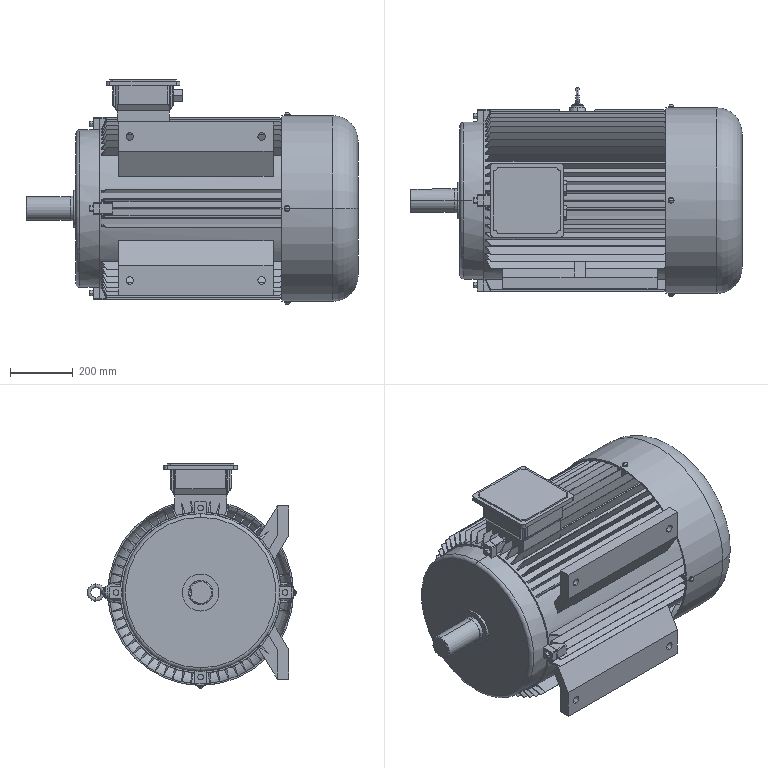Part | SolidWorks | features Boss 17, Cut 5, Revolution 5, Fillet 4, Chamfer 3, CirPattern 3, RevCut 2, 3DProfileFeature 1, LPattern 1, MirrorPattern 1, MoveCopyBody 1 | 2 solids | 614 faces | box 1055 x 665 x 715 mm | volume 197436858 mm3 | plane 377 | cone 138 | cylinder 79 | torus 12 | sphere 8 | commonest cylinder face diameters 16 x16 7.5 x12 18 x8 22.5 x8 24 x8 29.665 x4